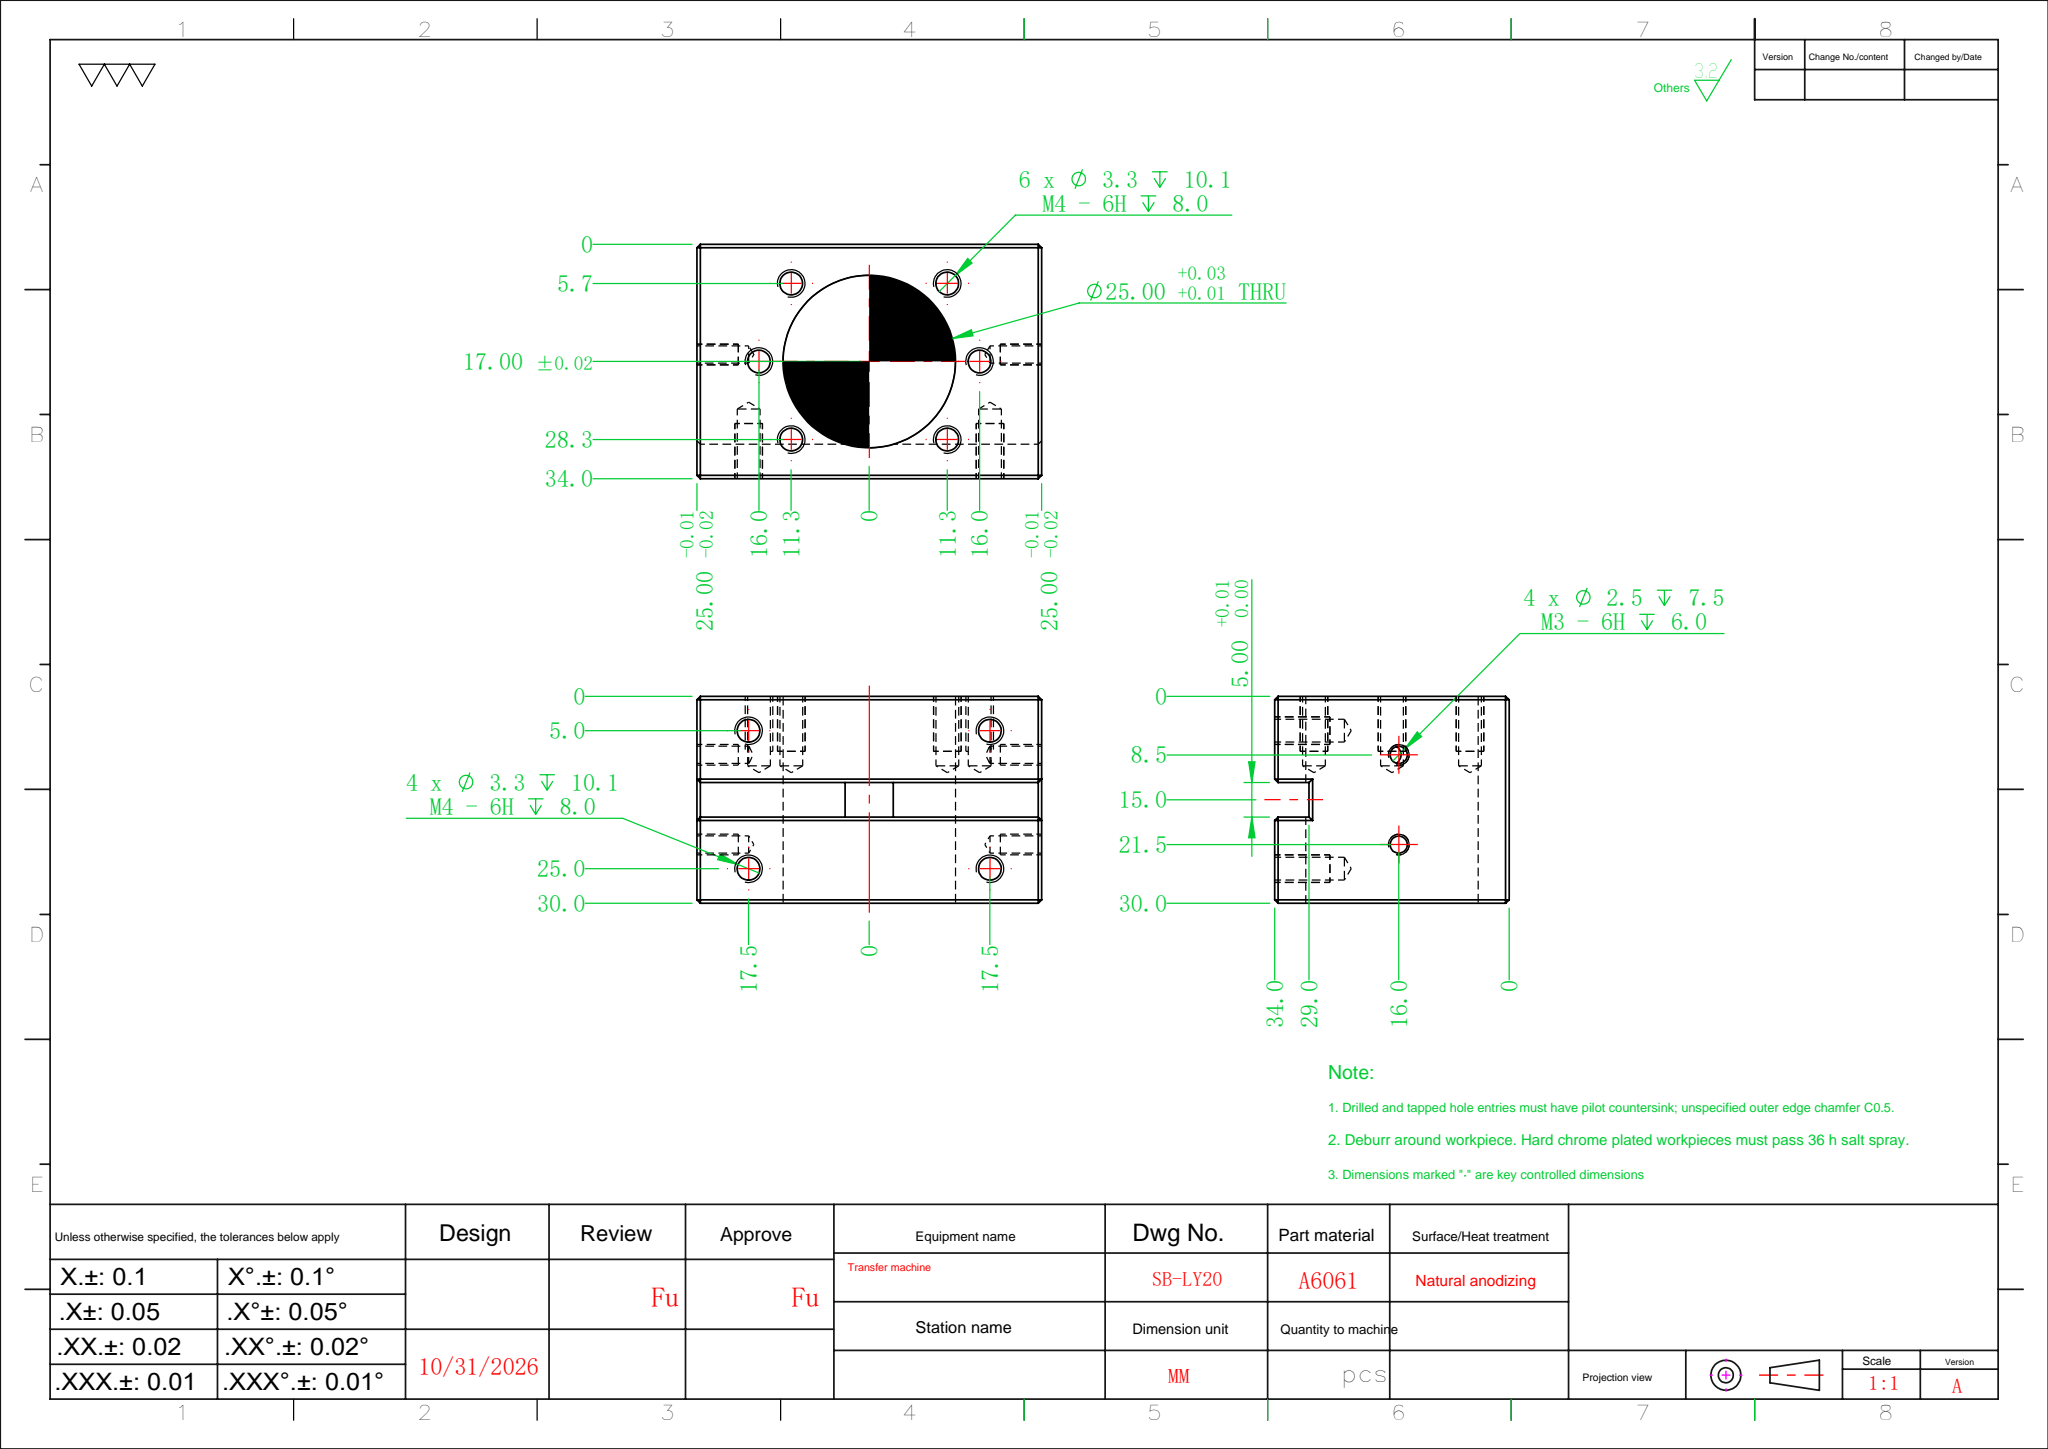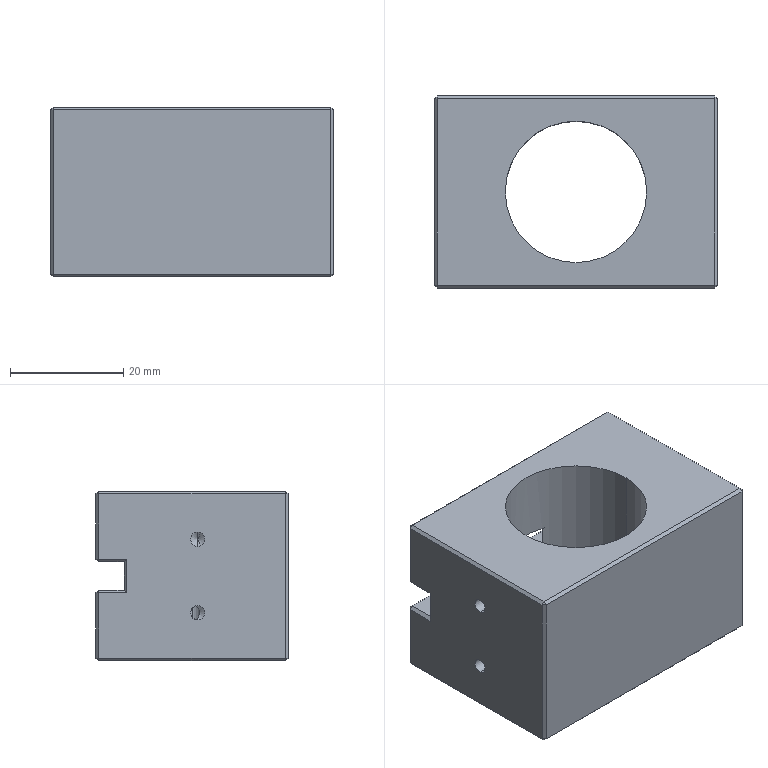Part | SolidWorks | features HoleWzd 3, Chamfer 1, Cut 1, Extrusion 1, ICE 1, MirrorPattern 1 | 1 solid | 105 faces | box 50 x 34 x 30 mm | volume 33922 mm3 | plane 45 | cylinder 30 | cone 30 | commonest cylinder face diameters 3.3 x20 2.5 x8 25 x2